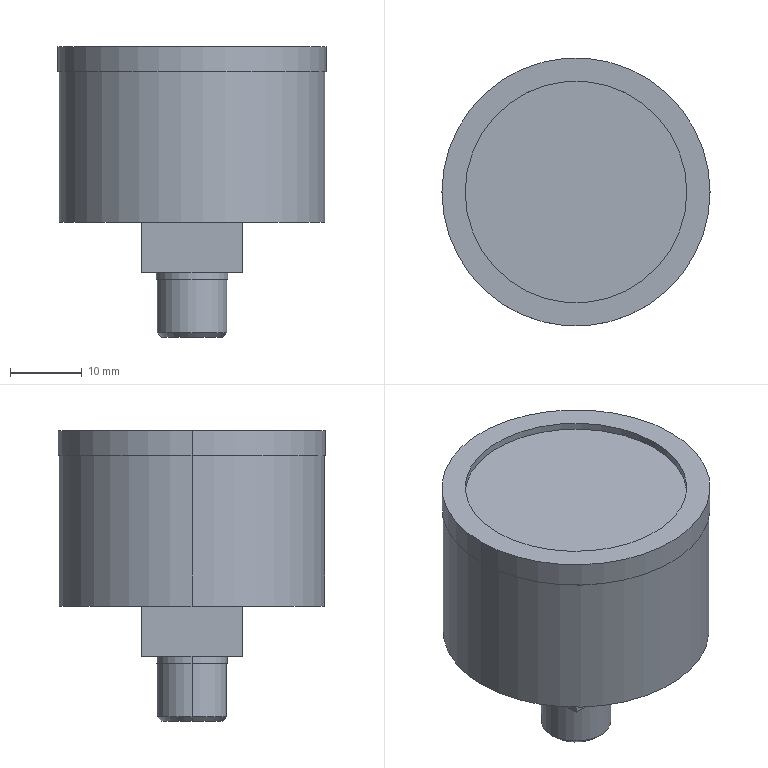Part | SolidWorks | features BaseBody 1 | 1 solid | 23 faces | box 37.5 x 37.5 x 40.6 mm | volume 27983 mm3 | plane 11 | cylinder 10 | cone 2 | commonest cylinder face diameters 9.728 x2 10 x2 31 x2 37.2 x2 37.5 x2
STEP:
#1=CARTESIAN_POINT('',(-4.283,0.,-9.1));
#2=VERTEX_POINT('',#1);
#3=CARTESIAN_POINT('',(4.283,0.,-9.1));
#4=VERTEX_POINT('',#3);
#5=CARTESIAN_POINT('',(0.,0.,-9.1));
#6=DIRECTION('',(0.,0.,-1.));
#7=DIRECTION('',(-1.,0.,0.));
#8=AXIS2_PLACEMENT_3D('',#5,#6,#7);
#9=CIRCLE('',#8,4.283);
#10=EDGE_CURVE('',#2,#4,#9,.T.);
#11=ORIENTED_EDGE('',*,*,#10,.F.);
#12=CARTESIAN_POINT('',(-4.864,0.,-8.519));
#13=VERTEX_POINT('',#12);
#14=CARTESIAN_POINT('',(-4.864,0.,-8.519));
#15=DIRECTION('',(-0.7071,0.,0.7071));
#16=VECTOR('',#15,1000.);
#17=LINE('',#14,#16);
#18=EDGE_CURVE('',#2,#13,#17,.T.);
#19=ORIENTED_EDGE('',*,*,#18,.T.);
#20=CARTESIAN_POINT('',(4.864,0.,-8.519));
#21=VERTEX_POINT('',#20);
#22=CARTESIAN_POINT('',(0.,0.,-8.519));
#23=DIRECTION('',(0.,0.,-1.));
#24=DIRECTION('',(-1.,0.,0.));
#25=AXIS2_PLACEMENT_3D('',#22,#23,#24);
#26=CIRCLE('',#25,4.864);
#27=EDGE_CURVE('',#13,#21,#26,.T.);
#28=ORIENTED_EDGE('',*,*,#27,.T.);
#29=CARTESIAN_POINT('',(4.864,0.,-8.519));
#30=DIRECTION('',(0.7071,0.,0.7071));
#31=VECTOR('',#30,1000.);
#32=LINE('',#29,#31);
#33=EDGE_CURVE('',#4,#21,#32,.T.);
#34=ORIENTED_EDGE('',*,*,#33,.F.);
#35=EDGE_LOOP('',(#11,#19,#28,#34));
#36=FACE_OUTER_BOUND('',#35,.T.);
#37=CARTESIAN_POINT('',(0.,0.,-8.519));
#38=DIRECTION('',(0.,0.,1.));
#39=DIRECTION('',(1.,0.,0.));
#40=AXIS2_PLACEMENT_3D('',#37,#38,#39);
#41=CONICAL_SURFACE('',#40,4.864,0.7854);
#42=ADVANCED_FACE('',(#36),#41,.T.);
#43=CARTESIAN_POINT('',(-4.864,0.,-1.));
#44=VERTEX_POINT('',#43);
#45=CARTESIAN_POINT('',(4.864,0.,-1.));
#46=VERTEX_POINT('',#45);
#47=CARTESIAN_POINT('',(0.,0.,-1.));
#48=DIRECTION('',(0.,0.,-1.));
#49=DIRECTION('',(-1.,0.,0.));
#50=AXIS2_PLACEMENT_3D('',#47,#48,#49);
#51=CIRCLE('',#50,4.864);
#52=EDGE_CURVE('',#44,#46,#51,.T.);
#53=ORIENTED_EDGE('',*,*,#52,.T.);
#54=CARTESIAN_POINT('',(4.864,0.,-9.1));
#55=DIRECTION('',(0.,0.,-1.));
#56=VECTOR('',#55,1000.);
#57=LINE('',#54,#56);
#58=EDGE_CURVE('',#46,#21,#57,.T.);
#59=ORIENTED_EDGE('',*,*,#58,.T.);
#60=ORIENTED_EDGE('',*,*,#27,.F.);
#61=CARTESIAN_POINT('',(-4.864,0.,-9.1));
#62=DIRECTION('',(0.,0.,-1.));
#63=VECTOR('',#62,1000.);
#64=LINE('',#61,#63);
#65=EDGE_CURVE('',#44,#13,#64,.T.);
#66=ORIENTED_EDGE('',*,*,#65,.F.);
#67=EDGE_LOOP('',(#53,#59,#60,#66));
#68=FACE_OUTER_BOUND('',#67,.T.);
#69=CARTESIAN_POINT('',(0.,0.,-9.1));
#70=DIRECTION('',(0.,0.,-1.));
#71=DIRECTION('',(-1.,0.,0.));
#72=AXIS2_PLACEMENT_3D('',#69,#70,#71);
#73=CYLINDRICAL_SURFACE('',#72,4.864);
#74=ADVANCED_FACE('',(#68),#73,.T.);
#75=CARTESIAN_POINT('',(-5.,0.,0.));
#76=VERTEX_POINT('',#75);
#77=CARTESIAN_POINT('',(5.,0.,0.));
#78=VERTEX_POINT('',#77);
#79=CARTESIAN_POINT('',(0.,0.,0.));
#80=DIRECTION('',(0.,0.,-1.));
#81=DIRECTION('',(-1.,0.,0.));
#82=AXIS2_PLACEMENT_3D('',#79,#80,#81);
#83=CIRCLE('',#82,5.);
#84=EDGE_CURVE('',#76,#78,#83,.T.);
#85=ORIENTED_EDGE('',*,*,#84,.T.);
#86=CARTESIAN_POINT('',(5.,0.,-1.));
#87=VERTEX_POINT('',#86);
#88=CARTESIAN_POINT('',(5.,0.,-9.1));
#89=DIRECTION('',(0.,0.,-1.));
#90=VECTOR('',#89,1000.);
#91=LINE('',#88,#90);
#92=EDGE_CURVE('',#78,#87,#91,.T.);
#93=ORIENTED_EDGE('',*,*,#92,.T.);
#94=CARTESIAN_POINT('',(-5.,0.,-1.));
#95=VERTEX_POINT('',#94);
#96=CARTESIAN_POINT('',(0.,0.,-1.));
#97=DIRECTION('',(0.,0.,-1.));
#98=DIRECTION('',(-1.,0.,0.));
#99=AXIS2_PLACEMENT_3D('',#96,#97,#98);
#100=CIRCLE('',#99,5.);
#101=EDGE_CURVE('',#95,#87,#100,.T.);
#102=ORIENTED_EDGE('',*,*,#101,.F.);
#103=CARTESIAN_POINT('',(-5.,0.,-9.1));
#104=DIRECTION('',(0.,0.,-1.));
#105=VECTOR('',#104,1000.);
#106=LINE('',#103,#105);
#107=EDGE_CURVE('',#76,#95,#106,.T.);
#108=ORIENTED_EDGE('',*,*,#107,.F.);
#109=EDGE_LOOP('',(#85,#93,#102,#108));
#110=FACE_OUTER_BOUND('',#109,.T.);
#111=CARTESIAN_POINT('',(0.,0.,-9.1));
#112=DIRECTION('',(0.,0.,-1.));
#113=DIRECTION('',(-1.,0.,0.));
#114=AXIS2_PLACEMENT_3D('',#111,#112,#113);
#115=CYLINDRICAL_SURFACE('',#114,5.);
#116=ADVANCED_FACE('',(#110),#115,.T.);
#117=CARTESIAN_POINT('',(-18.6,0.,28.));
#118=VERTEX_POINT('',#117);
#119=CARTESIAN_POINT('',(18.6,0.,28.));
#120=VERTEX_POINT('',#119);
#121=CARTESIAN_POINT('',(0.,0.,28.));
#122=DIRECTION('',(0.,0.,-1.));
#123=DIRECTION('',(-1.,0.,0.));
#124=AXIS2_PLACEMENT_3D('',#121,#122,#123);
#125=CIRCLE('',#124,18.6);
#126=EDGE_CURVE('',#118,#120,#125,.T.);
#127=ORIENTED_EDGE('',*,*,#126,.T.);
#128=CARTESIAN_POINT('',(18.6,0.,7.));
#129=VERTEX_POINT('',#128);
#130=CARTESIAN_POINT('',(18.6,0.,-9.1));
#131=DIRECTION('',(0.,0.,-1.));
#132=VECTOR('',#131,1000.);
#133=LINE('',#130,#132);
#134=EDGE_CURVE('',#120,#129,#133,.T.);
#135=ORIENTED_EDGE('',*,*,#134,.T.);
#136=CARTESIAN_POINT('',(-18.6,0.,7.));
#137=VERTEX_POINT('',#136);
#138=CARTESIAN_POINT('',(0.,0.,7.));
#139=DIRECTION('',(0.,0.,-1.));
#140=DIRECTION('',(-1.,0.,0.));
#141=AXIS2_PLACEMENT_3D('',#138,#139,#140);
#142=CIRCLE('',#141,18.6);
#143=EDGE_CURVE('',#137,#129,#142,.T.);
#144=ORIENTED_EDGE('',*,*,#143,.F.);
#145=CARTESIAN_POINT('',(-18.6,0.,-9.1));
#146=DIRECTION('',(0.,0.,-1.));
#147=VECTOR('',#146,1000.);
#148=LINE('',#145,#147);
#149=EDGE_CURVE('',#118,#137,#148,.T.);
#150=ORIENTED_EDGE('',*,*,#149,.F.);
#151=EDGE_LOOP('',(#127,#135,#144,#150));
#152=FACE_OUTER_BOUND('',#151,.T.);
#153=CARTESIAN_POINT('',(0.,0.,-9.1));
#154=DIRECTION('',(0.,0.,-1.));
#155=DIRECTION('',(-1.,0.,0.));
#156=AXIS2_PLACEMENT_3D('',#153,#154,#155);
#157=CYLINDRICAL_SURFACE('',#156,18.6);
#158=ADVANCED_FACE('',(#152),#157,.T.);
#159=CARTESIAN_POINT('',(-15.5,0.,30.5));
#160=VERTEX_POINT('',#159);
#161=CARTESIAN_POINT('',(15.5,0.,30.5));
#162=VERTEX_POINT('',#161);
#163=CARTESIAN_POINT('',(0.,0.,30.5));
#164=DIRECTION('',(0.,0.,1.));
#165=DIRECTION('',(0.,1.,0.));
#166=AXIS2_PLACEMENT_3D('',#163,#164,#165);
#167=CIRCLE('',#166,15.5);
#168=EDGE_CURVE('',#160,#162,#167,.T.);
#169=ORIENTED_EDGE('',*,*,#168,.F.);
#170=CARTESIAN_POINT('',(-15.5,0.,31.5));
#171=VERTEX_POINT('',#170);
#172=CARTESIAN_POINT('',(-15.5,0.,30.5));
#173=DIRECTION('',(0.,0.,1.));
#174=VECTOR('',#173,1000.);
#175=LINE('',#172,#174);
#176=EDGE_CURVE('',#160,#171,#175,.T.);
#177=ORIENTED_EDGE('',*,*,#176,.T.);
#178=CARTESIAN_POINT('',(15.5,0.,31.5));
#179=VERTEX_POINT('',#178);
#180=CARTESIAN_POINT('',(0.,0.,31.5));
#181=DIRECTION('',(0.,0.,1.));
#182=DIRECTION('',(0.,1.,0.));
#183=AXIS2_PLACEMENT_3D('',#180,#181,#182);
#184=CIRCLE('',#183,15.5);
#185=EDGE_CURVE('',#171,#179,#184,.T.);
#186=ORIENTED_EDGE('',*,*,#185,.T.);
#187=CARTESIAN_POINT('',(15.5,0.,30.5));
#188=DIRECTION('',(0.,0.,1.));
#189=VECTOR('',#188,1000.);
#190=LINE('',#187,#189);
#191=EDGE_CURVE('',#162,#179,#190,.T.);
#192=ORIENTED_EDGE('',*,*,#191,.F.);
#193=EDGE_LOOP('',(#169,#177,#186,#192));
#194=FACE_OUTER_BOUND('',#193,.T.);
#195=CARTESIAN_POINT('',(0.,0.,30.5));
#196=DIRECTION('',(0.,0.,1.));
#197=DIRECTION('',(1.,0.,0.));
#198=AXIS2_PLACEMENT_3D('',#195,#196,#197);
#199=CYLINDRICAL_SURFACE('',#198,15.5);
#200=ADVANCED_FACE('',(#194),#199,.F.);
#201=CARTESIAN_POINT('',(-18.75,0.,31.5));
#202=VERTEX_POINT('',#201);
#203=CARTESIAN_POINT('',(18.75,0.,31.5));
#204=VERTEX_POINT('',#203);
#205=CARTESIAN_POINT('',(0.,0.,31.5));
#206=DIRECTION('',(0.,0.,-1.));
#207=DIRECTION('',(-1.,0.,0.));
#208=AXIS2_PLACEMENT_3D('',#205,#206,#207);
#209=CIRCLE('',#208,18.75);
#210=EDGE_CURVE('',#202,#204,#209,.T.);
#211=ORIENTED_EDGE('',*,*,#210,.T.);
#212=CARTESIAN_POINT('',(18.75,0.,28.));
#213=VERTEX_POINT('',#212);
#214=CARTESIAN_POINT('',(18.75,0.,-9.1));
#215=DIRECTION('',(0.,0.,-1.));
#216=VECTOR('',#215,1000.);
#217=LINE('',#214,#216);
#218=EDGE_CURVE('',#204,#213,#217,.T.);
#219=ORIENTED_EDGE('',*,*,#218,.T.);
#220=CARTESIAN_POINT('',(-18.75,0.,28.));
#221=VERTEX_POINT('',#220);
#222=CARTESIAN_POINT('',(0.,0.,28.));
#223=DIRECTION('',(0.,0.,-1.));
#224=DIRECTION('',(-1.,0.,0.));
#225=AXIS2_PLACEMENT_3D('',#222,#223,#224);
#226=CIRCLE('',#225,18.75);
#227=EDGE_CURVE('',#221,#213,#226,.T.);
#228=ORIENTED_EDGE('',*,*,#227,.F.);
#229=CARTESIAN_POINT('',(-18.75,0.,-9.1));
#230=DIRECTION('',(0.,0.,-1.));
#231=VECTOR('',#230,1000.);
#232=LINE('',#229,#231);
#233=EDGE_CURVE('',#202,#221,#232,.T.);
#234=ORIENTED_EDGE('',*,*,#233,.F.);
#235=EDGE_LOOP('',(#211,#219,#228,#234));
#236=FACE_OUTER_BOUND('',#235,.T.);
#237=CARTESIAN_POINT('',(0.,0.,-9.1));
#238=DIRECTION('',(0.,0.,-1.));
#239=DIRECTION('',(-1.,0.,0.));
#240=AXIS2_PLACEMENT_3D('',#237,#238,#239);
#241=CYLINDRICAL_SURFACE('',#240,18.75);
#242=ADVANCED_FACE('',(#236),#241,.T.);
#243=ORIENTED_EDGE('',*,*,#210,.F.);
#244=CARTESIAN_POINT('',(0.,0.,31.5));
#245=DIRECTION('',(0.,0.,-1.));
#246=DIRECTION('',(-1.,0.,0.));
#247=AXIS2_PLACEMENT_3D('',#244,#245,#246);
#248=CIRCLE('',#247,18.75);
#249=EDGE_CURVE('',#204,#202,#248,.T.);
#250=ORIENTED_EDGE('',*,*,#249,.F.);
#251=EDGE_LOOP('',(#243,#250));
#252=FACE_OUTER_BOUND('',#251,.T.);
#253=CARTESIAN_POINT('',(0.,0.,31.5));
#254=DIRECTION('',(0.,0.,1.));
#255=DIRECTION('',(0.,1.,0.));
#256=AXIS2_PLACEMENT_3D('',#253,#254,#255);
#257=CIRCLE('',#256,15.5);
#258=EDGE_CURVE('',#179,#171,#257,.T.);
#259=ORIENTED_EDGE('',*,*,#258,.F.);
#260=ORIENTED_EDGE('',*,*,#185,.F.);
#261=EDGE_LOOP('',(#259,#260));
#262=FACE_BOUND('',#261,.T.);
#263=CARTESIAN_POINT('',(0.,0.,31.5));
#264=DIRECTION('',(0.,0.,-1.));
#265=DIRECTION('',(-1.,0.,0.));
#266=AXIS2_PLACEMENT_3D('',#263,#264,#265);
#267=PLANE('',#266);
#268=ADVANCED_FACE('',(#252,#262),#267,.F.);
#269=ORIENTED_EDGE('',*,*,#218,.F.);
#270=ORIENTED_EDGE('',*,*,#249,.T.);
#271=ORIENTED_EDGE('',*,*,#233,.T.);
#272=CARTESIAN_POINT('',(0.,0.,28.));
#273=DIRECTION('',(0.,0.,-1.));
#274=DIRECTION('',(-1.,0.,0.));
#275=AXIS2_PLACEMENT_3D('',#272,#273,#274);
#276=CIRCLE('',#275,18.75);
#277=EDGE_CURVE('',#213,#221,#276,.T.);
#278=ORIENTED_EDGE('',*,*,#277,.F.);
#279=EDGE_LOOP('',(#269,#270,#271,#278));
#280=FACE_OUTER_BOUND('',#279,.T.);
#281=CARTESIAN_POINT('',(0.,0.,-9.1));
#282=DIRECTION('',(0.,0.,-1.));
#283=DIRECTION('',(-1.,0.,0.));
#284=AXIS2_PLACEMENT_3D('',#281,#282,#283);
#285=CYLINDRICAL_SURFACE('',#284,18.75);
#286=ADVANCED_FACE('',(#280),#285,.T.);
#287=ORIENTED_EDGE('',*,*,#176,.F.);
#288=CARTESIAN_POINT('',(0.,0.,30.5));
#289=DIRECTION('',(0.,0.,1.));
#290=DIRECTION('',(0.,1.,0.));
#291=AXIS2_PLACEMENT_3D('',#288,#289,#290);
#292=CIRCLE('',#291,15.5);
#293=EDGE_CURVE('',#162,#160,#292,.T.);
#294=ORIENTED_EDGE('',*,*,#293,.F.);
#295=ORIENTED_EDGE('',*,*,#191,.T.);
#296=ORIENTED_EDGE('',*,*,#258,.T.);
#297=EDGE_LOOP('',(#287,#294,#295,#296));
#298=FACE_OUTER_BOUND('',#297,.T.);
#299=CARTESIAN_POINT('',(0.,0.,30.5));
#300=DIRECTION('',(0.,0.,1.));
#301=DIRECTION('',(1.,0.,0.));
#302=AXIS2_PLACEMENT_3D('',#299,#300,#301);
#303=CYLINDRICAL_SURFACE('',#302,15.5);
#304=ADVANCED_FACE('',(#298),#303,.F.);
#305=ORIENTED_EDGE('',*,*,#126,.F.);
#306=CARTESIAN_POINT('',(0.,0.,28.));
#307=DIRECTION('',(0.,0.,-1.));
#308=DIRECTION('',(-1.,0.,0.));
#309=AXIS2_PLACEMENT_3D('',#306,#307,#308);
#310=CIRCLE('',#309,18.6);
#311=EDGE_CURVE('',#120,#118,#310,.T.);
#312=ORIENTED_EDGE('',*,*,#311,.F.);
#313=EDGE_LOOP('',(#305,#312));
#314=FACE_BOUND('',#313,.T.);
#315=ORIENTED_EDGE('',*,*,#227,.T.);
#316=ORIENTED_EDGE('',*,*,#277,.T.);
#317=EDGE_LOOP('',(#315,#316));
#318=FACE_OUTER_BOUND('',#317,.T.);
#319=CARTESIAN_POINT('',(0.,18.75,28.));
#320=DIRECTION('',(0.,0.,1.));
#321=DIRECTION('',(1.,0.,0.));
#322=AXIS2_PLACEMENT_3D('',#319,#320,#321);
#323=PLANE('',#322);
#324=ADVANCED_FACE('',(#314,#318),#323,.F.);
#325=ORIENTED_EDGE('',*,*,#293,.T.);
#326=ORIENTED_EDGE('',*,*,#168,.T.);
#327=EDGE_LOOP('',(#325,#326));
#328=FACE_OUTER_BOUND('',#327,.T.);
#329=CARTESIAN_POINT('',(0.,0.,30.5));
#330=DIRECTION('',(0.,0.,1.));
#331=DIRECTION('',(1.,0.,0.));
#332=AXIS2_PLACEMENT_3D('',#329,#330,#331);
#333=PLANE('',#332);
#334=ADVANCED_FACE('',(#328),#333,.T.);
#335=ORIENTED_EDGE('',*,*,#134,.F.);
#336=ORIENTED_EDGE('',*,*,#311,.T.);
#337=ORIENTED_EDGE('',*,*,#149,.T.);
#338=CARTESIAN_POINT('',(0.,0.,7.));
#339=DIRECTION('',(0.,0.,-1.));
#340=DIRECTION('',(-1.,0.,0.));
#341=AXIS2_PLACEMENT_3D('',#338,#339,#340);
#342=CIRCLE('',#341,18.6);
#343=EDGE_CURVE('',#129,#137,#342,.T.);
#344=ORIENTED_EDGE('',*,*,#343,.F.);
#345=EDGE_LOOP('',(#335,#336,#337,#344));
#346=FACE_OUTER_BOUND('',#345,.T.);
#347=CARTESIAN_POINT('',(0.,0.,-9.1));
#348=DIRECTION('',(0.,0.,-1.));
#349=DIRECTION('',(-1.,0.,0.));
#350=AXIS2_PLACEMENT_3D('',#347,#348,#349);
#351=CYLINDRICAL_SURFACE('',#350,18.6);
#352=ADVANCED_FACE('',(#346),#351,.T.);
#353=ORIENTED_EDGE('',*,*,#143,.T.);
#354=ORIENTED_EDGE('',*,*,#343,.T.);
#355=EDGE_LOOP('',(#353,#354));
#356=FACE_OUTER_BOUND('',#355,.T.);
#357=CARTESIAN_POINT('',(7.,-7.,7.));
#358=VERTEX_POINT('',#357);
#359=CARTESIAN_POINT('',(-7.,-7.,7.));
#360=VERTEX_POINT('',#359);
#361=CARTESIAN_POINT('',(7.,-7.,7.));
#362=DIRECTION('',(-1.,0.,0.));
#363=VECTOR('',#362,1000.);
#364=LINE('',#361,#363);
#365=EDGE_CURVE('',#358,#360,#364,.T.);
#366=ORIENTED_EDGE('',*,*,#365,.F.);
#367=CARTESIAN_POINT('',(7.,7.,7.));
#368=VERTEX_POINT('',#367);
#369=CARTESIAN_POINT('',(7.,7.,7.));
#370=DIRECTION('',(0.,-1.,0.));
#371=VECTOR('',#370,1000.);
#372=LINE('',#369,#371);
#373=EDGE_CURVE('',#368,#358,#372,.T.);
#374=ORIENTED_EDGE('',*,*,#373,.F.);
#375=CARTESIAN_POINT('',(-7.,7.,7.));
#376=VERTEX_POINT('',#375);
#377=CARTESIAN_POINT('',(-7.,7.,7.));
#378=DIRECTION('',(1.,0.,0.));
#379=VECTOR('',#378,1000.);
#380=LINE('',#377,#379);
#381=EDGE_CURVE('',#376,#368,#380,.T.);
#382=ORIENTED_EDGE('',*,*,#381,.F.);
#383=CARTESIAN_POINT('',(-7.,-7.,7.));
#384=DIRECTION('',(0.,1.,0.));
#385=VECTOR('',#384,1000.);
#386=LINE('',#383,#385);
#387=EDGE_CURVE('',#360,#376,#386,.T.);
#388=ORIENTED_EDGE('',*,*,#387,.F.);
#389=EDGE_LOOP('',(#366,#374,#382,#388));
#390=FACE_BOUND('',#389,.T.);
#391=CARTESIAN_POINT('',(0.,18.6,7.));
#392=DIRECTION('',(0.,0.,1.));
#393=DIRECTION('',(1.,0.,0.));
#394=AXIS2_PLACEMENT_3D('',#391,#392,#393);
#395=PLANE('',#394);
#396=ADVANCED_FACE('',(#356,#390),#395,.F.);
#397=CARTESIAN_POINT('',(7.,-7.,0.));
#398=VERTEX_POINT('',#397);
#399=CARTESIAN_POINT('',(-7.,-7.,0.));
#400=VERTEX_POINT('',#399);
#401=CARTESIAN_POINT('',(7.,-7.,0.));
#402=DIRECTION('',(-1.,0.,0.));
#403=VECTOR('',#402,1000.);
#404=LINE('',#401,#403);
#405=EDGE_CURVE('',#398,#400,#404,.T.);
#406=ORIENTED_EDGE('',*,*,#405,.F.);
#407=CARTESIAN_POINT('',(7.,-7.,7.));
#408=DIRECTION('',(0.,0.,-1.));
#409=VECTOR('',#408,1000.);
#410=LINE('',#407,#409);
#411=EDGE_CURVE('',#358,#398,#410,.T.);
#412=ORIENTED_EDGE('',*,*,#411,.F.);
#413=ORIENTED_EDGE('',*,*,#365,.T.);
#414=CARTESIAN_POINT('',(-7.,-7.,7.));
#415=DIRECTION('',(0.,0.,-1.));
#416=VECTOR('',#415,1000.);
#417=LINE('',#414,#416);
#418=EDGE_CURVE('',#360,#400,#417,.T.);
#419=ORIENTED_EDGE('',*,*,#418,.T.);
#420=EDGE_LOOP('',(#406,#412,#413,#419));
#421=FACE_OUTER_BOUND('',#420,.T.);
#422=CARTESIAN_POINT('',(7.,-7.,7.));
#423=DIRECTION('',(0.,-1.,0.));
#424=DIRECTION('',(0.,0.,-1.));
#425=AXIS2_PLACEMENT_3D('',#422,#423,#424);
#426=PLANE('',#425);
#427=ADVANCED_FACE('',(#421),#426,.T.);
#428=CARTESIAN_POINT('',(7.,7.,0.));
#429=VERTEX_POINT('',#428);
#430=CARTESIAN_POINT('',(7.,7.,0.));
#431=DIRECTION('',(0.,-1.,0.));
#432=VECTOR('',#431,1000.);
#433=LINE('',#430,#432);
#434=EDGE_CURVE('',#429,#398,#433,.T.);
#435=ORIENTED_EDGE('',*,*,#434,.F.);
#436=CARTESIAN_POINT('',(7.,7.,7.));
#437=DIRECTION('',(0.,0.,-1.));
#438=VECTOR('',#437,1000.);
#439=LINE('',#436,#438);
#440=EDGE_CURVE('',#368,#429,#439,.T.);
#441=ORIENTED_EDGE('',*,*,#440,.F.);
#442=ORIENTED_EDGE('',*,*,#373,.T.);
#443=ORIENTED_EDGE('',*,*,#411,.T.);
#444=EDGE_LOOP('',(#435,#441,#442,#443));
#445=FACE_OUTER_BOUND('',#444,.T.);
#446=CARTESIAN_POINT('',(7.,7.,7.));
#447=DIRECTION('',(1.,0.,0.));
#448=DIRECTION('',(0.,0.,-1.));
#449=AXIS2_PLACEMENT_3D('',#446,#447,#448);
#450=PLANE('',#449);
#451=ADVANCED_FACE('',(#445),#450,.T.);
#452=CARTESIAN_POINT('',(-7.,7.,0.));
#453=VERTEX_POINT('',#452);
#454=CARTESIAN_POINT('',(7.,7.,0.));
#455=DIRECTION('',(-1.,0.,0.));
#456=VECTOR('',#455,1000.);
#457=LINE('',#454,#456);
#458=EDGE_CURVE('',#429,#453,#457,.T.);
#459=ORIENTED_EDGE('',*,*,#458,.T.);
#460=CARTESIAN_POINT('',(-7.,7.,7.));
#461=DIRECTION('',(0.,0.,-1.));
#462=VECTOR('',#461,1000.);
#463=LINE('',#460,#462);
#464=EDGE_CURVE('',#376,#453,#463,.T.);
#465=ORIENTED_EDGE('',*,*,#464,.F.);
#466=ORIENTED_EDGE('',*,*,#381,.T.);
#467=ORIENTED_EDGE('',*,*,#440,.T.);
#468=EDGE_LOOP('',(#459,#465,#466,#467));
#469=FACE_OUTER_BOUND('',#468,.T.);
#470=CARTESIAN_POINT('',(-7.,7.,7.));
#471=DIRECTION('',(0.,1.,0.));
#472=DIRECTION('',(0.,0.,1.));
#473=AXIS2_PLACEMENT_3D('',#470,#471,#472);
#474=PLANE('',#473);
#475=ADVANCED_FACE('',(#469),#474,.T.);
#476=CARTESIAN_POINT('',(-7.,-7.,0.));
#477=DIRECTION('',(0.,1.,0.));
#478=VECTOR('',#477,1000.);
#479=LINE('',#476,#478);
#480=EDGE_CURVE('',#400,#453,#479,.T.);
#481=ORIENTED_EDGE('',*,*,#480,.F.);
#482=ORIENTED_EDGE('',*,*,#418,.F.);
#483=ORIENTED_EDGE('',*,*,#387,.T.);
#484=ORIENTED_EDGE('',*,*,#464,.T.);
#485=EDGE_LOOP('',(#481,#482,#483,#484));
#486=FACE_OUTER_BOUND('',#485,.T.);
#487=CARTESIAN_POINT('',(-7.,-7.,7.));
#488=DIRECTION('',(-1.,0.,0.));
#489=DIRECTION('',(0.,0.,1.));
#490=AXIS2_PLACEMENT_3D('',#487,#488,#489);
#491=PLANE('',#490);
#492=ADVANCED_FACE('',(#486),#491,.T.);
#493=ORIENTED_EDGE('',*,*,#84,.F.);
#494=CARTESIAN_POINT('',(0.,0.,0.));
#495=DIRECTION('',(0.,0.,-1.));
#496=DIRECTION('',(-1.,0.,0.));
#497=AXIS2_PLACEMENT_3D('',#494,#495,#496);
#498=CIRCLE('',#497,5.);
#499=EDGE_CURVE('',#78,#76,#498,.T.);
#500=ORIENTED_EDGE('',*,*,#499,.F.);
#501=EDGE_LOOP('',(#493,#500));
#502=FACE_BOUND('',#501,.T.);
#503=ORIENTED_EDGE('',*,*,#405,.T.);
#504=ORIENTED_EDGE('',*,*,#480,.T.);
#505=ORIENTED_EDGE('',*,*,#458,.F.);
#506=ORIENTED_EDGE('',*,*,#434,.T.);
#507=EDGE_LOOP('',(#503,#504,#505,#506));
#508=FACE_OUTER_BOUND('',#507,.T.);
#509=CARTESIAN_POINT('',(0.,15.,0.));
#510=DIRECTION('',(0.,0.,1.));
#511=DIRECTION('',(1.,0.,0.));
#512=AXIS2_PLACEMENT_3D('',#509,#510,#511);
#513=PLANE('',#512);
#514=ADVANCED_FACE('',(#502,#508),#513,.F.);
#515=ORIENTED_EDGE('',*,*,#92,.F.);
#516=ORIENTED_EDGE('',*,*,#499,.T.);
#517=ORIENTED_EDGE('',*,*,#107,.T.);
#518=CARTESIAN_POINT('',(0.,0.,-1.));
#519=DIRECTION('',(0.,0.,-1.));
#520=DIRECTION('',(-1.,0.,0.));
#521=AXIS2_PLACEMENT_3D('',#518,#519,#520);
#522=CIRCLE('',#521,5.);
#523=EDGE_CURVE('',#87,#95,#522,.T.);
#524=ORIENTED_EDGE('',*,*,#523,.F.);
#525=EDGE_LOOP('',(#515,#516,#517,#524));
#526=FACE_OUTER_BOUND('',#525,.T.);
#527=CARTESIAN_POINT('',(0.,0.,-9.1));
#528=DIRECTION('',(0.,0.,-1.));
#529=DIRECTION('',(-1.,0.,0.));
#530=AXIS2_PLACEMENT_3D('',#527,#528,#529);
#531=CYLINDRICAL_SURFACE('',#530,5.);
#532=ADVANCED_FACE('',(#526),#531,.T.);
#533=ORIENTED_EDGE('',*,*,#52,.F.);
#534=CARTESIAN_POINT('',(0.,0.,-1.));
#535=DIRECTION('',(0.,0.,-1.));
#536=DIRECTION('',(-1.,0.,0.));
#537=AXIS2_PLACEMENT_3D('',#534,#535,#536);
#538=CIRCLE('',#537,4.864);
#539=EDGE_CURVE('',#46,#44,#538,.T.);
#540=ORIENTED_EDGE('',*,*,#539,.F.);
#541=EDGE_LOOP('',(#533,#540));
#542=FACE_BOUND('',#541,.T.);
#543=ORIENTED_EDGE('',*,*,#101,.T.);
#544=ORIENTED_EDGE('',*,*,#523,.T.);
#545=EDGE_LOOP('',(#543,#544));
#546=FACE_OUTER_BOUND('',#545,.T.);
#547=CARTESIAN_POINT('',(0.,5.,-1.));
#548=DIRECTION('',(0.,0.,1.));
#549=DIRECTION('',(1.,0.,0.));
#550=AXIS2_PLACEMENT_3D('',#547,#548,#549);
#551=PLANE('',#550);
#552=ADVANCED_FACE('',(#542,#546),#551,.F.);
#553=ORIENTED_EDGE('',*,*,#58,.F.);
#554=ORIENTED_EDGE('',*,*,#539,.T.);
#555=ORIENTED_EDGE('',*,*,#65,.T.);
#556=CARTESIAN_POINT('',(0.,0.,-8.519));
#557=DIRECTION('',(0.,0.,-1.));
#558=DIRECTION('',(-1.,0.,0.));
#559=AXIS2_PLACEMENT_3D('',#556,#557,#558);
#560=CIRCLE('',#559,4.864);
#561=EDGE_CURVE('',#21,#13,#560,.T.);
#562=ORIENTED_EDGE('',*,*,#561,.F.);
#563=EDGE_LOOP('',(#553,#554,#555,#562));
#564=FACE_OUTER_BOUND('',#563,.T.);
#565=CARTESIAN_POINT('',(0.,0.,-9.1));
#566=DIRECTION('',(0.,0.,-1.));
#567=DIRECTION('',(-1.,0.,0.));
#568=AXIS2_PLACEMENT_3D('',#565,#566,#567);
#569=CYLINDRICAL_SURFACE('',#568,4.864);
#570=ADVANCED_FACE('',(#564),#569,.T.);
#571=ORIENTED_EDGE('',*,*,#18,.F.);
#572=CARTESIAN_POINT('',(0.,0.,-9.1));
#573=DIRECTION('',(0.,0.,-1.));
#574=DIRECTION('',(-1.,0.,0.));
#575=AXIS2_PLACEMENT_3D('',#572,#573,#574);
#576=CIRCLE('',#575,4.283);
#577=EDGE_CURVE('',#4,#2,#576,.T.);
#578=ORIENTED_EDGE('',*,*,#577,.F.);
#579=ORIENTED_EDGE('',*,*,#33,.T.);
#580=ORIENTED_EDGE('',*,*,#561,.T.);
#581=EDGE_LOOP('',(#571,#578,#579,#580));
#582=FACE_OUTER_BOUND('',#581,.T.);
#583=CARTESIAN_POINT('',(0.,0.,-8.519));
#584=DIRECTION('',(0.,0.,1.));
#585=DIRECTION('',(1.,0.,0.));
#586=AXIS2_PLACEMENT_3D('',#583,#584,#585);
#587=CONICAL_SURFACE('',#586,4.864,0.7854);
#588=ADVANCED_FACE('',(#582),#587,.T.);
#589=ORIENTED_EDGE('',*,*,#577,.T.);
#590=ORIENTED_EDGE('',*,*,#10,.T.);
#591=EDGE_LOOP('',(#589,#590));
#592=FACE_OUTER_BOUND('',#591,.T.);
#593=CARTESIAN_POINT('',(0.,4.283,-9.1));
#594=DIRECTION('',(0.,0.,1.));
#595=DIRECTION('',(1.,0.,0.));
#596=AXIS2_PLACEMENT_3D('',#593,#594,#595);
#597=PLANE('',#596);
#598=ADVANCED_FACE('',(#592),#597,.F.);
#599=CLOSED_SHELL('',(#42,#74,#116,#158,#200,#242,#268,#286,#304,#324,#334,#352,#396,#427,#451,#475,#492,#514,#532,#552,#570,#588,#598));
#600=MANIFOLD_SOLID_BREP('',#599);
#601=CARTESIAN_POINT('',(0.,0.,0.));
#602=DIRECTION('',(0.,0.,1.));
#603=DIRECTION('',(1.,0.,0.));
#604=AXIS2_PLACEMENT_3D('',#601,#602,#603);
#605=(LENGTH_UNIT()NAMED_UNIT(*)SI_UNIT(.MILLI.,.METRE.));
#606=UNCERTAINTY_MEASURE_WITH_UNIT(LENGTH_MEASURE(0.00001),#605,'','');
#607=(NAMED_UNIT(*)PLANE_ANGLE_UNIT()SI_UNIT($,.RADIAN.));
#608=(NAMED_UNIT(*)SI_UNIT($,.STERADIAN.)SOLID_ANGLE_UNIT());
#609=(GEOMETRIC_REPRESENTATION_CONTEXT(3)GLOBAL_UNCERTAINTY_ASSIGNED_CONTEXT((#606))GLOBAL_UNIT_ASSIGNED_CONTEXT((#605,#607,#608))REPRESENTATION_CONTEXT('',''));
#610=ADVANCED_BREP_SHAPE_REPRESENTATION('',(#600,#604),#609);